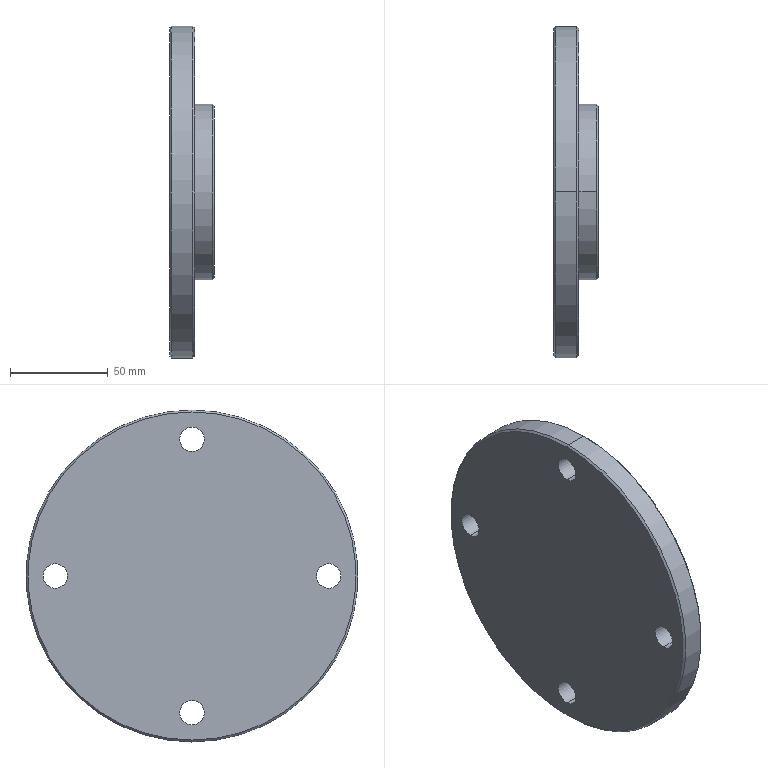Part | SolidWorks | features Chamfer 1, CirPattern 1, ICE 1, Revolution 1 | 1 solid | 26 faces | box 23 x 170 x 170 mm | volume 323268 mm3 | cylinder 14 | cone 8 | plane 4 | commonest cylinder face diameters 12.5 x8 60 x2 90 x2 170 x2
STEP:
#1=CARTESIAN_POINT('',(13.,0.,-84.));
#2=VERTEX_POINT('',#1);
#3=CARTESIAN_POINT('',(13.,0.,84.));
#4=VERTEX_POINT('',#3);
#5=CARTESIAN_POINT('',(13.,0.,0.));
#6=DIRECTION('',(1.,0.,0.));
#7=DIRECTION('',(0.,0.,1.));
#8=AXIS2_PLACEMENT_3D('',#5,#6,#7);
#9=CIRCLE('',#8,84.);
#10=EDGE_CURVE('',#2,#4,#9,.T.);
#11=ORIENTED_EDGE('',*,*,#10,.F.);
#12=CARTESIAN_POINT('',(12.,0.,-85.));
#13=VERTEX_POINT('',#12);
#14=CARTESIAN_POINT('',(12.,0.,-85.));
#15=DIRECTION('',(-0.7071,0.,-0.7071));
#16=VECTOR('',#15,1000.);
#17=LINE('',#14,#16);
#18=EDGE_CURVE('',#2,#13,#17,.T.);
#19=ORIENTED_EDGE('',*,*,#18,.T.);
#20=CARTESIAN_POINT('',(12.,0.,85.));
#21=VERTEX_POINT('',#20);
#22=CARTESIAN_POINT('',(12.,0.,0.));
#23=DIRECTION('',(-1.,0.,0.));
#24=DIRECTION('',(0.,0.,1.));
#25=AXIS2_PLACEMENT_3D('',#22,#23,#24);
#26=CIRCLE('',#25,85.);
#27=EDGE_CURVE('',#21,#13,#26,.T.);
#28=ORIENTED_EDGE('',*,*,#27,.F.);
#29=CARTESIAN_POINT('',(12.,0.,85.));
#30=DIRECTION('',(-0.7071,0.,0.7071));
#31=VECTOR('',#30,1000.);
#32=LINE('',#29,#31);
#33=EDGE_CURVE('',#4,#21,#32,.T.);
#34=ORIENTED_EDGE('',*,*,#33,.F.);
#35=EDGE_LOOP('',(#11,#19,#28,#34));
#36=FACE_OUTER_BOUND('',#35,.T.);
#37=CARTESIAN_POINT('',(12.,0.,0.));
#38=DIRECTION('',(-1.,0.,0.));
#39=DIRECTION('',(0.,0.,1.));
#40=AXIS2_PLACEMENT_3D('',#37,#38,#39);
#41=CONICAL_SURFACE('',#40,85.,0.7854);
#42=ADVANCED_FACE('',(#36),#41,.T.);
#43=CARTESIAN_POINT('',(0.,0.,84.));
#44=VERTEX_POINT('',#43);
#45=CARTESIAN_POINT('',(0.,0.,-84.));
#46=VERTEX_POINT('',#45);
#47=CARTESIAN_POINT('',(0.,0.,0.));
#48=DIRECTION('',(-1.,0.,0.));
#49=DIRECTION('',(0.,0.,-1.));
#50=AXIS2_PLACEMENT_3D('',#47,#48,#49);
#51=CIRCLE('',#50,84.);
#52=EDGE_CURVE('',#44,#46,#51,.T.);
#53=ORIENTED_EDGE('',*,*,#52,.F.);
#54=CARTESIAN_POINT('',(1.,0.,85.));
#55=VERTEX_POINT('',#54);
#56=CARTESIAN_POINT('',(0.,0.,84.));
#57=DIRECTION('',(0.7071,0.,0.7071));
#58=VECTOR('',#57,1000.);
#59=LINE('',#56,#58);
#60=EDGE_CURVE('',#44,#55,#59,.T.);
#61=ORIENTED_EDGE('',*,*,#60,.T.);
#62=CARTESIAN_POINT('',(1.,0.,-85.));
#63=VERTEX_POINT('',#62);
#64=CARTESIAN_POINT('',(1.,0.,0.));
#65=DIRECTION('',(1.,0.,0.));
#66=DIRECTION('',(0.,0.,-1.));
#67=AXIS2_PLACEMENT_3D('',#64,#65,#66);
#68=CIRCLE('',#67,85.);
#69=EDGE_CURVE('',#63,#55,#68,.T.);
#70=ORIENTED_EDGE('',*,*,#69,.F.);
#71=CARTESIAN_POINT('',(0.,0.,-84.));
#72=DIRECTION('',(0.7071,0.,-0.7071));
#73=VECTOR('',#72,1000.);
#74=LINE('',#71,#73);
#75=EDGE_CURVE('',#46,#63,#74,.T.);
#76=ORIENTED_EDGE('',*,*,#75,.F.);
#77=EDGE_LOOP('',(#53,#61,#70,#76));
#78=FACE_OUTER_BOUND('',#77,.T.);
#79=CARTESIAN_POINT('',(0.,0.,0.));
#80=DIRECTION('',(1.,0.,0.));
#81=DIRECTION('',(0.,0.,-1.));
#82=AXIS2_PLACEMENT_3D('',#79,#80,#81);
#83=CONICAL_SURFACE('',#82,84.,0.7854);
#84=ADVANCED_FACE('',(#78),#83,.T.);
#85=CARTESIAN_POINT('',(23.,0.,-44.));
#86=VERTEX_POINT('',#85);
#87=CARTESIAN_POINT('',(23.,0.,44.));
#88=VERTEX_POINT('',#87);
#89=CARTESIAN_POINT('',(23.,0.,0.));
#90=DIRECTION('',(1.,0.,0.));
#91=DIRECTION('',(0.,0.,1.));
#92=AXIS2_PLACEMENT_3D('',#89,#90,#91);
#93=CIRCLE('',#92,44.);
#94=EDGE_CURVE('',#86,#88,#93,.T.);
#95=ORIENTED_EDGE('',*,*,#94,.F.);
#96=CARTESIAN_POINT('',(22.,0.,-45.));
#97=VERTEX_POINT('',#96);
#98=CARTESIAN_POINT('',(22.,0.,-45.));
#99=DIRECTION('',(-0.7071,0.,-0.7071));
#100=VECTOR('',#99,1000.);
#101=LINE('',#98,#100);
#102=EDGE_CURVE('',#86,#97,#101,.T.);
#103=ORIENTED_EDGE('',*,*,#102,.T.);
#104=CARTESIAN_POINT('',(22.,0.,45.));
#105=VERTEX_POINT('',#104);
#106=CARTESIAN_POINT('',(22.,0.,0.));
#107=DIRECTION('',(-1.,0.,0.));
#108=DIRECTION('',(0.,0.,1.));
#109=AXIS2_PLACEMENT_3D('',#106,#107,#108);
#110=CIRCLE('',#109,45.);
#111=EDGE_CURVE('',#105,#97,#110,.T.);
#112=ORIENTED_EDGE('',*,*,#111,.F.);
#113=CARTESIAN_POINT('',(22.,0.,45.));
#114=DIRECTION('',(-0.7071,0.,0.7071));
#115=VECTOR('',#114,1000.);
#116=LINE('',#113,#115);
#117=EDGE_CURVE('',#88,#105,#116,.T.);
#118=ORIENTED_EDGE('',*,*,#117,.F.);
#119=EDGE_LOOP('',(#95,#103,#112,#118));
#120=FACE_OUTER_BOUND('',#119,.T.);
#121=CARTESIAN_POINT('',(22.,0.,0.));
#122=DIRECTION('',(-1.,0.,0.));
#123=DIRECTION('',(0.,0.,1.));
#124=AXIS2_PLACEMENT_3D('',#121,#122,#123);
#125=CONICAL_SURFACE('',#124,45.,0.7854);
#126=ADVANCED_FACE('',(#120),#125,.T.);
#127=CARTESIAN_POINT('',(22.,0.,30.));
#128=VERTEX_POINT('',#127);
#129=CARTESIAN_POINT('',(22.,0.,-30.));
#130=VERTEX_POINT('',#129);
#131=CARTESIAN_POINT('',(22.,0.,0.));
#132=DIRECTION('',(1.,0.,0.));
#133=DIRECTION('',(0.,0.,1.));
#134=AXIS2_PLACEMENT_3D('',#131,#132,#133);
#135=CIRCLE('',#134,30.);
#136=EDGE_CURVE('',#128,#130,#135,.T.);
#137=ORIENTED_EDGE('',*,*,#136,.F.);
#138=CARTESIAN_POINT('',(23.,0.,31.));
#139=VERTEX_POINT('',#138);
#140=CARTESIAN_POINT('',(23.,0.,31.));
#141=DIRECTION('',(0.7071,0.,0.7071));
#142=VECTOR('',#141,1000.);
#143=LINE('',#140,#142);
#144=EDGE_CURVE('',#128,#139,#143,.T.);
#145=ORIENTED_EDGE('',*,*,#144,.T.);
#146=CARTESIAN_POINT('',(23.,0.,-31.));
#147=VERTEX_POINT('',#146);
#148=CARTESIAN_POINT('',(23.,0.,0.));
#149=DIRECTION('',(-1.,0.,0.));
#150=DIRECTION('',(0.,0.,1.));
#151=AXIS2_PLACEMENT_3D('',#148,#149,#150);
#152=CIRCLE('',#151,31.);
#153=EDGE_CURVE('',#147,#139,#152,.T.);
#154=ORIENTED_EDGE('',*,*,#153,.F.);
#155=CARTESIAN_POINT('',(23.,0.,-31.));
#156=DIRECTION('',(0.7071,0.,-0.7071));
#157=VECTOR('',#156,1000.);
#158=LINE('',#155,#157);
#159=EDGE_CURVE('',#130,#147,#158,.T.);
#160=ORIENTED_EDGE('',*,*,#159,.F.);
#161=EDGE_LOOP('',(#137,#145,#154,#160));
#162=FACE_OUTER_BOUND('',#161,.T.);
#163=CARTESIAN_POINT('',(23.,0.,0.));
#164=DIRECTION('',(1.,0.,0.));
#165=DIRECTION('',(0.,0.,-1.));
#166=AXIS2_PLACEMENT_3D('',#163,#164,#165);
#167=CONICAL_SURFACE('',#166,31.,0.7854);
#168=ADVANCED_FACE('',(#162),#167,.F.);
#169=CARTESIAN_POINT('',(13.,-70.,-6.25));
#170=VERTEX_POINT('',#169);
#171=CARTESIAN_POINT('',(13.,-70.,6.25));
#172=VERTEX_POINT('',#171);
#173=CARTESIAN_POINT('',(13.,-70.,0.));
#174=DIRECTION('',(-1.,0.,0.));
#175=DIRECTION('',(0.,0.,1.));
#176=AXIS2_PLACEMENT_3D('',#173,#174,#175);
#177=CIRCLE('',#176,6.25);
#178=EDGE_CURVE('',#170,#172,#177,.T.);
#179=ORIENTED_EDGE('',*,*,#178,.F.);
#180=CARTESIAN_POINT('',(0.,-70.,-6.25));
#181=VERTEX_POINT('',#180);
#182=CARTESIAN_POINT('',(23.,-70.,-6.25));
#183=DIRECTION('',(-1.,0.,0.));
#184=VECTOR('',#183,1000.);
#185=LINE('',#182,#184);
#186=EDGE_CURVE('',#170,#181,#185,.T.);
#187=ORIENTED_EDGE('',*,*,#186,.T.);
#188=CARTESIAN_POINT('',(0.,-70.,6.25));
#189=VERTEX_POINT('',#188);
#190=CARTESIAN_POINT('',(0.,-70.,0.));
#191=DIRECTION('',(-1.,0.,0.));
#192=DIRECTION('',(0.,0.,-1.));
#193=AXIS2_PLACEMENT_3D('',#190,#191,#192);
#194=CIRCLE('',#193,6.25);
#195=EDGE_CURVE('',#181,#189,#194,.T.);
#196=ORIENTED_EDGE('',*,*,#195,.T.);
#197=CARTESIAN_POINT('',(23.,-70.,6.25));
#198=DIRECTION('',(-1.,0.,0.));
#199=VECTOR('',#198,1000.);
#200=LINE('',#197,#199);
#201=EDGE_CURVE('',#172,#189,#200,.T.);
#202=ORIENTED_EDGE('',*,*,#201,.F.);
#203=EDGE_LOOP('',(#179,#187,#196,#202));
#204=FACE_OUTER_BOUND('',#203,.T.);
#205=CARTESIAN_POINT('',(23.,-70.,0.));
#206=DIRECTION('',(-1.,0.,0.));
#207=DIRECTION('',(0.,0.,1.));
#208=AXIS2_PLACEMENT_3D('',#205,#206,#207);
#209=CYLINDRICAL_SURFACE('',#208,6.25);
#210=ADVANCED_FACE('',(#204),#209,.F.);
#211=CARTESIAN_POINT('',(13.,0.,63.75));
#212=VERTEX_POINT('',#211);
#213=CARTESIAN_POINT('',(13.,0.,76.25));
#214=VERTEX_POINT('',#213);
#215=CARTESIAN_POINT('',(13.,0.,70.));
#216=DIRECTION('',(-1.,0.,0.));
#217=DIRECTION('',(0.,0.,1.));
#218=AXIS2_PLACEMENT_3D('',#215,#216,#217);
#219=CIRCLE('',#218,6.25);
#220=EDGE_CURVE('',#212,#214,#219,.T.);
#221=ORIENTED_EDGE('',*,*,#220,.F.);
#222=CARTESIAN_POINT('',(0.,0.,63.75));
#223=VERTEX_POINT('',#222);
#224=CARTESIAN_POINT('',(23.,0.,63.75));
#225=DIRECTION('',(-1.,0.,0.));
#226=VECTOR('',#225,1000.);
#227=LINE('',#224,#226);
#228=EDGE_CURVE('',#212,#223,#227,.T.);
#229=ORIENTED_EDGE('',*,*,#228,.T.);
#230=CARTESIAN_POINT('',(0.,0.,76.25));
#231=VERTEX_POINT('',#230);
#232=CARTESIAN_POINT('',(0.,0.,70.));
#233=DIRECTION('',(-1.,0.,0.));
#234=DIRECTION('',(0.,-1.,0.));
#235=AXIS2_PLACEMENT_3D('',#232,#233,#234);
#236=CIRCLE('',#235,6.25);
#237=EDGE_CURVE('',#223,#231,#236,.T.);
#238=ORIENTED_EDGE('',*,*,#237,.T.);
#239=CARTESIAN_POINT('',(23.,0.,76.25));
#240=DIRECTION('',(-1.,0.,0.));
#241=VECTOR('',#240,1000.);
#242=LINE('',#239,#241);
#243=EDGE_CURVE('',#214,#231,#242,.T.);
#244=ORIENTED_EDGE('',*,*,#243,.F.);
#245=EDGE_LOOP('',(#221,#229,#238,#244));
#246=FACE_OUTER_BOUND('',#245,.T.);
#247=CARTESIAN_POINT('',(23.,0.,70.));
#248=DIRECTION('',(-1.,0.,0.));
#249=DIRECTION('',(0.,0.,1.));
#250=AXIS2_PLACEMENT_3D('',#247,#248,#249);
#251=CYLINDRICAL_SURFACE('',#250,6.25);
#252=ADVANCED_FACE('',(#246),#251,.F.);
#253=CARTESIAN_POINT('',(13.,0.,-76.25));
#254=VERTEX_POINT('',#253);
#255=CARTESIAN_POINT('',(13.,0.,-63.75));
#256=VERTEX_POINT('',#255);
#257=CARTESIAN_POINT('',(13.,0.,-70.));
#258=DIRECTION('',(-1.,0.,0.));
#259=DIRECTION('',(0.,0.,1.));
#260=AXIS2_PLACEMENT_3D('',#257,#258,#259);
#261=CIRCLE('',#260,6.25);
#262=EDGE_CURVE('',#254,#256,#261,.T.);
#263=ORIENTED_EDGE('',*,*,#262,.F.);
#264=CARTESIAN_POINT('',(0.,0.,-76.25));
#265=VERTEX_POINT('',#264);
#266=CARTESIAN_POINT('',(23.,0.,-76.25));
#267=DIRECTION('',(-1.,0.,0.));
#268=VECTOR('',#267,1000.);
#269=LINE('',#266,#268);
#270=EDGE_CURVE('',#254,#265,#269,.T.);
#271=ORIENTED_EDGE('',*,*,#270,.T.);
#272=CARTESIAN_POINT('',(0.,0.,-63.75));
#273=VERTEX_POINT('',#272);
#274=CARTESIAN_POINT('',(0.,0.,-70.));
#275=DIRECTION('',(-1.,0.,0.));
#276=DIRECTION('',(0.,1.,0.));
#277=AXIS2_PLACEMENT_3D('',#274,#275,#276);
#278=CIRCLE('',#277,6.25);
#279=EDGE_CURVE('',#265,#273,#278,.T.);
#280=ORIENTED_EDGE('',*,*,#279,.T.);
#281=CARTESIAN_POINT('',(23.,0.,-63.75));
#282=DIRECTION('',(-1.,0.,0.));
#283=VECTOR('',#282,1000.);
#284=LINE('',#281,#283);
#285=EDGE_CURVE('',#256,#273,#284,.T.);
#286=ORIENTED_EDGE('',*,*,#285,.F.);
#287=EDGE_LOOP('',(#263,#271,#280,#286));
#288=FACE_OUTER_BOUND('',#287,.T.);
#289=CARTESIAN_POINT('',(23.,0.,-70.));
#290=DIRECTION('',(-1.,0.,0.));
#291=DIRECTION('',(0.,0.,1.));
#292=AXIS2_PLACEMENT_3D('',#289,#290,#291);
#293=CYLINDRICAL_SURFACE('',#292,6.25);
#294=ADVANCED_FACE('',(#288),#293,.F.);
#295=CARTESIAN_POINT('',(13.,70.,-6.25));
#296=VERTEX_POINT('',#295);
#297=CARTESIAN_POINT('',(13.,70.,6.25));
#298=VERTEX_POINT('',#297);
#299=CARTESIAN_POINT('',(13.,70.,0.));
#300=DIRECTION('',(-1.,0.,0.));
#301=DIRECTION('',(0.,0.,1.));
#302=AXIS2_PLACEMENT_3D('',#299,#300,#301);
#303=CIRCLE('',#302,6.25);
#304=EDGE_CURVE('',#296,#298,#303,.T.);
#305=ORIENTED_EDGE('',*,*,#304,.F.);
#306=CARTESIAN_POINT('',(0.,70.,-6.25));
#307=VERTEX_POINT('',#306);
#308=CARTESIAN_POINT('',(23.,70.,-6.25));
#309=DIRECTION('',(-1.,0.,0.));
#310=VECTOR('',#309,1000.);
#311=LINE('',#308,#310);
#312=EDGE_CURVE('',#296,#307,#311,.T.);
#313=ORIENTED_EDGE('',*,*,#312,.T.);
#314=CARTESIAN_POINT('',(0.,70.,6.25));
#315=VERTEX_POINT('',#314);
#316=CARTESIAN_POINT('',(0.,70.,0.));
#317=DIRECTION('',(-1.,0.,0.));
#318=DIRECTION('',(0.,0.,1.));
#319=AXIS2_PLACEMENT_3D('',#316,#317,#318);
#320=CIRCLE('',#319,6.25);
#321=EDGE_CURVE('',#307,#315,#320,.T.);
#322=ORIENTED_EDGE('',*,*,#321,.T.);
#323=CARTESIAN_POINT('',(23.,70.,6.25));
#324=DIRECTION('',(-1.,0.,0.));
#325=VECTOR('',#324,1000.);
#326=LINE('',#323,#325);
#327=EDGE_CURVE('',#298,#315,#326,.T.);
#328=ORIENTED_EDGE('',*,*,#327,.F.);
#329=EDGE_LOOP('',(#305,#313,#322,#328));
#330=FACE_OUTER_BOUND('',#329,.T.);
#331=CARTESIAN_POINT('',(23.,70.,0.));
#332=DIRECTION('',(-1.,0.,0.));
#333=DIRECTION('',(0.,0.,1.));
#334=AXIS2_PLACEMENT_3D('',#331,#332,#333);
#335=CYLINDRICAL_SURFACE('',#334,6.25);
#336=ADVANCED_FACE('',(#330),#335,.F.);
#337=ORIENTED_EDGE('',*,*,#136,.T.);
#338=CARTESIAN_POINT('',(13.,0.,-30.));
#339=VERTEX_POINT('',#338);
#340=CARTESIAN_POINT('',(0.,0.,-30.));
#341=DIRECTION('',(-1.,0.,0.));
#342=VECTOR('',#341,1000.);
#343=LINE('',#340,#342);
#344=EDGE_CURVE('',#130,#339,#343,.T.);
#345=ORIENTED_EDGE('',*,*,#344,.T.);
#346=CARTESIAN_POINT('',(13.,0.,30.));
#347=VERTEX_POINT('',#346);
#348=CARTESIAN_POINT('',(13.,0.,0.));
#349=DIRECTION('',(-1.,0.,0.));
#350=DIRECTION('',(0.,0.,1.));
#351=AXIS2_PLACEMENT_3D('',#348,#349,#350);
#352=CIRCLE('',#351,30.);
#353=EDGE_CURVE('',#339,#347,#352,.T.);
#354=ORIENTED_EDGE('',*,*,#353,.T.);
#355=CARTESIAN_POINT('',(0.,0.,30.));
#356=DIRECTION('',(-1.,0.,0.));
#357=VECTOR('',#356,1000.);
#358=LINE('',#355,#357);
#359=EDGE_CURVE('',#128,#347,#358,.T.);
#360=ORIENTED_EDGE('',*,*,#359,.F.);
#361=EDGE_LOOP('',(#337,#345,#354,#360));
#362=FACE_OUTER_BOUND('',#361,.T.);
#363=CARTESIAN_POINT('',(0.,0.,0.));
#364=DIRECTION('',(-1.,0.,0.));
#365=DIRECTION('',(0.,0.,1.));
#366=AXIS2_PLACEMENT_3D('',#363,#364,#365);
#367=CYLINDRICAL_SURFACE('',#366,30.);
#368=ADVANCED_FACE('',(#362),#367,.F.);
#369=ORIENTED_EDGE('',*,*,#111,.T.);
#370=CARTESIAN_POINT('',(13.,0.,-45.));
#371=VERTEX_POINT('',#370);
#372=CARTESIAN_POINT('',(0.,0.,-45.));
#373=DIRECTION('',(-1.,0.,0.));
#374=VECTOR('',#373,1000.);
#375=LINE('',#372,#374);
#376=EDGE_CURVE('',#97,#371,#375,.T.);
#377=ORIENTED_EDGE('',*,*,#376,.T.);
#378=CARTESIAN_POINT('',(13.,0.,45.));
#379=VERTEX_POINT('',#378);
#380=CARTESIAN_POINT('',(13.,0.,0.));
#381=DIRECTION('',(-1.,0.,0.));
#382=DIRECTION('',(0.,0.,1.));
#383=AXIS2_PLACEMENT_3D('',#380,#381,#382);
#384=CIRCLE('',#383,45.);
#385=EDGE_CURVE('',#379,#371,#384,.T.);
#386=ORIENTED_EDGE('',*,*,#385,.F.);
#387=CARTESIAN_POINT('',(0.,0.,45.));
#388=DIRECTION('',(-1.,0.,0.));
#389=VECTOR('',#388,1000.);
#390=LINE('',#387,#389);
#391=EDGE_CURVE('',#105,#379,#390,.T.);
#392=ORIENTED_EDGE('',*,*,#391,.F.);
#393=EDGE_LOOP('',(#369,#377,#386,#392));
#394=FACE_OUTER_BOUND('',#393,.T.);
#395=CARTESIAN_POINT('',(0.,0.,0.));
#396=DIRECTION('',(-1.,0.,0.));
#397=DIRECTION('',(0.,0.,1.));
#398=AXIS2_PLACEMENT_3D('',#395,#396,#397);
#399=CYLINDRICAL_SURFACE('',#398,45.);
#400=ADVANCED_FACE('',(#394),#399,.T.);
#401=ORIENTED_EDGE('',*,*,#27,.T.);
#402=CARTESIAN_POINT('',(0.,0.,-85.));
#403=DIRECTION('',(-1.,0.,0.));
#404=VECTOR('',#403,1000.);
#405=LINE('',#402,#404);
#406=EDGE_CURVE('',#13,#63,#405,.T.);
#407=ORIENTED_EDGE('',*,*,#406,.T.);
#408=ORIENTED_EDGE('',*,*,#69,.T.);
#409=CARTESIAN_POINT('',(0.,0.,85.));
#410=DIRECTION('',(-1.,0.,0.));
#411=VECTOR('',#410,1000.);
#412=LINE('',#409,#411);
#413=EDGE_CURVE('',#21,#55,#412,.T.);
#414=ORIENTED_EDGE('',*,*,#413,.F.);
#415=EDGE_LOOP('',(#401,#407,#408,#414));
#416=FACE_OUTER_BOUND('',#415,.T.);
#417=CARTESIAN_POINT('',(0.,0.,0.));
#418=DIRECTION('',(-1.,0.,0.));
#419=DIRECTION('',(0.,0.,1.));
#420=AXIS2_PLACEMENT_3D('',#417,#418,#419);
#421=CYLINDRICAL_SURFACE('',#420,85.);
#422=ADVANCED_FACE('',(#416),#421,.T.);
#423=CARTESIAN_POINT('',(0.,0.,0.));
#424=DIRECTION('',(-1.,0.,0.));
#425=DIRECTION('',(0.,0.,-1.));
#426=AXIS2_PLACEMENT_3D('',#423,#424,#425);
#427=CIRCLE('',#426,84.);
#428=EDGE_CURVE('',#46,#44,#427,.T.);
#429=ORIENTED_EDGE('',*,*,#428,.T.);
#430=ORIENTED_EDGE('',*,*,#52,.T.);
#431=EDGE_LOOP('',(#429,#430));
#432=FACE_OUTER_BOUND('',#431,.T.);
#433=CARTESIAN_POINT('',(0.,-70.,0.));
#434=DIRECTION('',(-1.,0.,0.));
#435=DIRECTION('',(0.,0.,-1.));
#436=AXIS2_PLACEMENT_3D('',#433,#434,#435);
#437=CIRCLE('',#436,6.25);
#438=EDGE_CURVE('',#189,#181,#437,.T.);
#439=ORIENTED_EDGE('',*,*,#438,.F.);
#440=ORIENTED_EDGE('',*,*,#195,.F.);
#441=EDGE_LOOP('',(#439,#440));
#442=FACE_BOUND('',#441,.T.);
#443=CARTESIAN_POINT('',(0.,0.,70.));
#444=DIRECTION('',(-1.,0.,0.));
#445=DIRECTION('',(0.,-1.,0.));
#446=AXIS2_PLACEMENT_3D('',#443,#444,#445);
#447=CIRCLE('',#446,6.25);
#448=EDGE_CURVE('',#231,#223,#447,.T.);
#449=ORIENTED_EDGE('',*,*,#448,.F.);
#450=ORIENTED_EDGE('',*,*,#237,.F.);
#451=EDGE_LOOP('',(#449,#450));
#452=FACE_BOUND('',#451,.T.);
#453=CARTESIAN_POINT('',(0.,0.,-70.));
#454=DIRECTION('',(-1.,0.,0.));
#455=DIRECTION('',(0.,1.,0.));
#456=AXIS2_PLACEMENT_3D('',#453,#454,#455);
#457=CIRCLE('',#456,6.25);
#458=EDGE_CURVE('',#273,#265,#457,.T.);
#459=ORIENTED_EDGE('',*,*,#458,.F.);
#460=ORIENTED_EDGE('',*,*,#279,.F.);
#461=EDGE_LOOP('',(#459,#460));
#462=FACE_BOUND('',#461,.T.);
#463=CARTESIAN_POINT('',(0.,70.,0.));
#464=DIRECTION('',(-1.,0.,0.));
#465=DIRECTION('',(0.,0.,1.));
#466=AXIS2_PLACEMENT_3D('',#463,#464,#465);
#467=CIRCLE('',#466,6.25);
#468=EDGE_CURVE('',#315,#307,#467,.T.);
#469=ORIENTED_EDGE('',*,*,#468,.F.);
#470=ORIENTED_EDGE('',*,*,#321,.F.);
#471=EDGE_LOOP('',(#469,#470));
#472=FACE_BOUND('',#471,.T.);
#473=CARTESIAN_POINT('',(0.,0.,0.));
#474=DIRECTION('',(1.,0.,0.));
#475=DIRECTION('',(0.,0.,-1.));
#476=AXIS2_PLACEMENT_3D('',#473,#474,#475);
#477=PLANE('',#476);
#478=ADVANCED_FACE('',(#432,#442,#452,#462,#472),#477,.F.);
#479=ORIENTED_EDGE('',*,*,#406,.F.);
#480=CARTESIAN_POINT('',(12.,0.,0.));
#481=DIRECTION('',(-1.,0.,0.));
#482=DIRECTION('',(0.,0.,1.));
#483=AXIS2_PLACEMENT_3D('',#480,#481,#482);
#484=CIRCLE('',#483,85.);
#485=EDGE_CURVE('',#13,#21,#484,.T.);
#486=ORIENTED_EDGE('',*,*,#485,.T.);
#487=ORIENTED_EDGE('',*,*,#413,.T.);
#488=CARTESIAN_POINT('',(1.,0.,0.));
#489=DIRECTION('',(1.,0.,0.));
#490=DIRECTION('',(0.,0.,-1.));
#491=AXIS2_PLACEMENT_3D('',#488,#489,#490);
#492=CIRCLE('',#491,85.);
#493=EDGE_CURVE('',#55,#63,#492,.T.);
#494=ORIENTED_EDGE('',*,*,#493,.T.);
#495=EDGE_LOOP('',(#479,#486,#487,#494));
#496=FACE_OUTER_BOUND('',#495,.T.);
#497=CARTESIAN_POINT('',(0.,0.,0.));
#498=DIRECTION('',(-1.,0.,0.));
#499=DIRECTION('',(0.,0.,1.));
#500=AXIS2_PLACEMENT_3D('',#497,#498,#499);
#501=CYLINDRICAL_SURFACE('',#500,85.);
#502=ADVANCED_FACE('',(#496),#501,.T.);
#503=CARTESIAN_POINT('',(13.,0.,0.));
#504=DIRECTION('',(1.,0.,0.));
#505=DIRECTION('',(0.,0.,1.));
#506=AXIS2_PLACEMENT_3D('',#503,#504,#505);
#507=CIRCLE('',#506,84.);
#508=EDGE_CURVE('',#4,#2,#507,.T.);
#509=ORIENTED_EDGE('',*,*,#508,.T.);
#510=ORIENTED_EDGE('',*,*,#10,.T.);
#511=EDGE_LOOP('',(#509,#510));
#512=FACE_OUTER_BOUND('',#511,.T.);
#513=CARTESIAN_POINT('',(13.,-70.,0.));
#514=DIRECTION('',(-1.,0.,0.));
#515=DIRECTION('',(0.,0.,1.));
#516=AXIS2_PLACEMENT_3D('',#513,#514,#515);
#517=CIRCLE('',#516,6.25);
#518=EDGE_CURVE('',#172,#170,#517,.T.);
#519=ORIENTED_EDGE('',*,*,#518,.T.);
#520=ORIENTED_EDGE('',*,*,#178,.T.);
#521=EDGE_LOOP('',(#519,#520));
#522=FACE_BOUND('',#521,.T.);
#523=CARTESIAN_POINT('',(13.,0.,70.));
#524=DIRECTION('',(-1.,0.,0.));
#525=DIRECTION('',(0.,0.,1.));
#526=AXIS2_PLACEMENT_3D('',#523,#524,#525);
#527=CIRCLE('',#526,6.25);
#528=EDGE_CURVE('',#214,#212,#527,.T.);
#529=ORIENTED_EDGE('',*,*,#528,.T.);
#530=ORIENTED_EDGE('',*,*,#220,.T.);
#531=EDGE_LOOP('',(#529,#530));
#532=FACE_BOUND('',#531,.T.);
#533=CARTESIAN_POINT('',(13.,0.,-70.));
#534=DIRECTION('',(-1.,0.,0.));
#535=DIRECTION('',(0.,0.,1.));
#536=AXIS2_PLACEMENT_3D('',#533,#534,#535);
#537=CIRCLE('',#536,6.25);
#538=EDGE_CURVE('',#256,#254,#537,.T.);
#539=ORIENTED_EDGE('',*,*,#538,.T.);
#540=ORIENTED_EDGE('',*,*,#262,.T.);
#541=EDGE_LOOP('',(#539,#540));
#542=FACE_BOUND('',#541,.T.);
#543=CARTESIAN_POINT('',(13.,70.,0.));
#544=DIRECTION('',(-1.,0.,0.));
#545=DIRECTION('',(0.,0.,1.));
#546=AXIS2_PLACEMENT_3D('',#543,#544,#545);
#547=CIRCLE('',#546,6.25);
#548=EDGE_CURVE('',#298,#296,#547,.T.);
#549=ORIENTED_EDGE('',*,*,#548,.T.);
#550=ORIENTED_EDGE('',*,*,#304,.T.);
#551=EDGE_LOOP('',(#549,#550));
#552=FACE_BOUND('',#551,.T.);
#553=ORIENTED_EDGE('',*,*,#385,.T.);
#554=CARTESIAN_POINT('',(13.,0.,0.));
#555=DIRECTION('',(-1.,0.,0.));
#556=DIRECTION('',(0.,0.,1.));
#557=AXIS2_PLACEMENT_3D('',#554,#555,#556);
#558=CIRCLE('',#557,45.);
#559=EDGE_CURVE('',#371,#379,#558,.T.);
#560=ORIENTED_EDGE('',*,*,#559,.T.);
#561=EDGE_LOOP('',(#553,#560));
#562=FACE_BOUND('',#561,.T.);
#563=CARTESIAN_POINT('',(13.,85.,0.));
#564=DIRECTION('',(-1.,0.,0.));
#565=DIRECTION('',(0.,0.,1.));
#566=AXIS2_PLACEMENT_3D('',#563,#564,#565);
#567=PLANE('',#566);
#568=ADVANCED_FACE('',(#512,#522,#532,#542,#552,#562),#567,.F.);
#569=ORIENTED_EDGE('',*,*,#376,.F.);
#570=CARTESIAN_POINT('',(22.,0.,0.));
#571=DIRECTION('',(-1.,0.,0.));
#572=DIRECTION('',(0.,0.,1.));
#573=AXIS2_PLACEMENT_3D('',#570,#571,#572);
#574=CIRCLE('',#573,45.);
#575=EDGE_CURVE('',#97,#105,#574,.T.);
#576=ORIENTED_EDGE('',*,*,#575,.T.);
#577=ORIENTED_EDGE('',*,*,#391,.T.);
#578=ORIENTED_EDGE('',*,*,#559,.F.);
#579=EDGE_LOOP('',(#569,#576,#577,#578));
#580=FACE_OUTER_BOUND('',#579,.T.);
#581=CARTESIAN_POINT('',(0.,0.,0.));
#582=DIRECTION('',(-1.,0.,0.));
#583=DIRECTION('',(0.,0.,1.));
#584=AXIS2_PLACEMENT_3D('',#581,#582,#583);
#585=CYLINDRICAL_SURFACE('',#584,45.);
#586=ADVANCED_FACE('',(#580),#585,.T.);
#587=ORIENTED_EDGE('',*,*,#153,.T.);
#588=CARTESIAN_POINT('',(23.,0.,0.));
#589=DIRECTION('',(-1.,0.,0.));
#590=DIRECTION('',(0.,0.,1.));
#591=AXIS2_PLACEMENT_3D('',#588,#589,#590);
#592=CIRCLE('',#591,31.);
#593=EDGE_CURVE('',#139,#147,#592,.T.);
#594=ORIENTED_EDGE('',*,*,#593,.T.);
#595=EDGE_LOOP('',(#587,#594));
#596=FACE_BOUND('',#595,.T.);
#597=CARTESIAN_POINT('',(23.,0.,0.));
#598=DIRECTION('',(1.,0.,0.));
#599=DIRECTION('',(0.,0.,1.));
#600=AXIS2_PLACEMENT_3D('',#597,#598,#599);
#601=CIRCLE('',#600,44.);
#602=EDGE_CURVE('',#88,#86,#601,.T.);
#603=ORIENTED_EDGE('',*,*,#602,.T.);
#604=ORIENTED_EDGE('',*,*,#94,.T.);
#605=EDGE_LOOP('',(#603,#604));
#606=FACE_OUTER_BOUND('',#605,.T.);
#607=CARTESIAN_POINT('',(23.,45.,0.));
#608=DIRECTION('',(-1.,0.,0.));
#609=DIRECTION('',(0.,0.,1.));
#610=AXIS2_PLACEMENT_3D('',#607,#608,#609);
#611=PLANE('',#610);
#612=ADVANCED_FACE('',(#596,#606),#611,.F.);
#613=ORIENTED_EDGE('',*,*,#344,.F.);
#614=CARTESIAN_POINT('',(22.,0.,0.));
#615=DIRECTION('',(1.,0.,0.));
#616=DIRECTION('',(0.,0.,1.));
#617=AXIS2_PLACEMENT_3D('',#614,#615,#616);
#618=CIRCLE('',#617,30.);
#619=EDGE_CURVE('',#130,#128,#618,.T.);
#620=ORIENTED_EDGE('',*,*,#619,.T.);
#621=ORIENTED_EDGE('',*,*,#359,.T.);
#622=CARTESIAN_POINT('',(13.,0.,0.));
#623=DIRECTION('',(-1.,0.,0.));
#624=DIRECTION('',(0.,0.,1.));
#625=AXIS2_PLACEMENT_3D('',#622,#623,#624);
#626=CIRCLE('',#625,30.);
#627=EDGE_CURVE('',#347,#339,#626,.T.);
#628=ORIENTED_EDGE('',*,*,#627,.T.);
#629=EDGE_LOOP('',(#613,#620,#621,#628));
#630=FACE_OUTER_BOUND('',#629,.T.);
#631=CARTESIAN_POINT('',(0.,0.,0.));
#632=DIRECTION('',(-1.,0.,0.));
#633=DIRECTION('',(0.,0.,1.));
#634=AXIS2_PLACEMENT_3D('',#631,#632,#633);
#635=CYLINDRICAL_SURFACE('',#634,30.);
#636=ADVANCED_FACE('',(#630),#635,.F.);
#637=ORIENTED_EDGE('',*,*,#627,.F.);
#638=ORIENTED_EDGE('',*,*,#353,.F.);
#639=EDGE_LOOP('',(#637,#638));
#640=FACE_OUTER_BOUND('',#639,.T.);
#641=CARTESIAN_POINT('',(13.,30.,0.));
#642=DIRECTION('',(-1.,0.,0.));
#643=DIRECTION('',(0.,0.,1.));
#644=AXIS2_PLACEMENT_3D('',#641,#642,#643);
#645=PLANE('',#644);
#646=ADVANCED_FACE('',(#640),#645,.F.);
#647=ORIENTED_EDGE('',*,*,#312,.F.);
#648=ORIENTED_EDGE('',*,*,#548,.F.);
#649=ORIENTED_EDGE('',*,*,#327,.T.);
#650=ORIENTED_EDGE('',*,*,#468,.T.);
#651=EDGE_LOOP('',(#647,#648,#649,#650));
#652=FACE_OUTER_BOUND('',#651,.T.);
#653=CARTESIAN_POINT('',(23.,70.,0.));
#654=DIRECTION('',(-1.,0.,0.));
#655=DIRECTION('',(0.,0.,1.));
#656=AXIS2_PLACEMENT_3D('',#653,#654,#655);
#657=CYLINDRICAL_SURFACE('',#656,6.25);
#658=ADVANCED_FACE('',(#652),#657,.F.);
#659=ORIENTED_EDGE('',*,*,#270,.F.);
#660=ORIENTED_EDGE('',*,*,#538,.F.);
#661=ORIENTED_EDGE('',*,*,#285,.T.);
#662=ORIENTED_EDGE('',*,*,#458,.T.);
#663=EDGE_LOOP('',(#659,#660,#661,#662));
#664=FACE_OUTER_BOUND('',#663,.T.);
#665=CARTESIAN_POINT('',(23.,0.,-70.));
#666=DIRECTION('',(-1.,0.,0.));
#667=DIRECTION('',(0.,0.,1.));
#668=AXIS2_PLACEMENT_3D('',#665,#666,#667);
#669=CYLINDRICAL_SURFACE('',#668,6.25);
#670=ADVANCED_FACE('',(#664),#669,.F.);
#671=ORIENTED_EDGE('',*,*,#228,.F.);
#672=ORIENTED_EDGE('',*,*,#528,.F.);
#673=ORIENTED_EDGE('',*,*,#243,.T.);
#674=ORIENTED_EDGE('',*,*,#448,.T.);
#675=EDGE_LOOP('',(#671,#672,#673,#674));
#676=FACE_OUTER_BOUND('',#675,.T.);
#677=CARTESIAN_POINT('',(23.,0.,70.));
#678=DIRECTION('',(-1.,0.,0.));
#679=DIRECTION('',(0.,0.,1.));
#680=AXIS2_PLACEMENT_3D('',#677,#678,#679);
#681=CYLINDRICAL_SURFACE('',#680,6.25);
#682=ADVANCED_FACE('',(#676),#681,.F.);
#683=ORIENTED_EDGE('',*,*,#186,.F.);
#684=ORIENTED_EDGE('',*,*,#518,.F.);
#685=ORIENTED_EDGE('',*,*,#201,.T.);
#686=ORIENTED_EDGE('',*,*,#438,.T.);
#687=EDGE_LOOP('',(#683,#684,#685,#686));
#688=FACE_OUTER_BOUND('',#687,.T.);
#689=CARTESIAN_POINT('',(23.,-70.,0.));
#690=DIRECTION('',(-1.,0.,0.));
#691=DIRECTION('',(0.,0.,1.));
#692=AXIS2_PLACEMENT_3D('',#689,#690,#691);
#693=CYLINDRICAL_SURFACE('',#692,6.25);
#694=ADVANCED_FACE('',(#688),#693,.F.);
#695=ORIENTED_EDGE('',*,*,#144,.F.);
#696=ORIENTED_EDGE('',*,*,#619,.F.);
#697=ORIENTED_EDGE('',*,*,#159,.T.);
#698=ORIENTED_EDGE('',*,*,#593,.F.);
#699=EDGE_LOOP('',(#695,#696,#697,#698));
#700=FACE_OUTER_BOUND('',#699,.T.);
#701=CARTESIAN_POINT('',(23.,0.,0.));
#702=DIRECTION('',(1.,0.,0.));
#703=DIRECTION('',(0.,0.,-1.));
#704=AXIS2_PLACEMENT_3D('',#701,#702,#703);
#705=CONICAL_SURFACE('',#704,31.,0.7854);
#706=ADVANCED_FACE('',(#700),#705,.F.);
#707=ORIENTED_EDGE('',*,*,#102,.F.);
#708=ORIENTED_EDGE('',*,*,#602,.F.);
#709=ORIENTED_EDGE('',*,*,#117,.T.);
#710=ORIENTED_EDGE('',*,*,#575,.F.);
#711=EDGE_LOOP('',(#707,#708,#709,#710));
#712=FACE_OUTER_BOUND('',#711,.T.);
#713=CARTESIAN_POINT('',(22.,0.,0.));
#714=DIRECTION('',(-1.,0.,0.));
#715=DIRECTION('',(0.,0.,1.));
#716=AXIS2_PLACEMENT_3D('',#713,#714,#715);
#717=CONICAL_SURFACE('',#716,45.,0.7854);
#718=ADVANCED_FACE('',(#712),#717,.T.);
#719=ORIENTED_EDGE('',*,*,#60,.F.);
#720=ORIENTED_EDGE('',*,*,#428,.F.);
#721=ORIENTED_EDGE('',*,*,#75,.T.);
#722=ORIENTED_EDGE('',*,*,#493,.F.);
#723=EDGE_LOOP('',(#719,#720,#721,#722));
#724=FACE_OUTER_BOUND('',#723,.T.);
#725=CARTESIAN_POINT('',(0.,0.,0.));
#726=DIRECTION('',(1.,0.,0.));
#727=DIRECTION('',(0.,0.,-1.));
#728=AXIS2_PLACEMENT_3D('',#725,#726,#727);
#729=CONICAL_SURFACE('',#728,84.,0.7854);
#730=ADVANCED_FACE('',(#724),#729,.T.);
#731=ORIENTED_EDGE('',*,*,#18,.F.);
#732=ORIENTED_EDGE('',*,*,#508,.F.);
#733=ORIENTED_EDGE('',*,*,#33,.T.);
#734=ORIENTED_EDGE('',*,*,#485,.F.);
#735=EDGE_LOOP('',(#731,#732,#733,#734));
#736=FACE_OUTER_BOUND('',#735,.T.);
#737=CARTESIAN_POINT('',(12.,0.,0.));
#738=DIRECTION('',(-1.,0.,0.));
#739=DIRECTION('',(0.,0.,1.));
#740=AXIS2_PLACEMENT_3D('',#737,#738,#739);
#741=CONICAL_SURFACE('',#740,85.,0.7854);
#742=ADVANCED_FACE('',(#736),#741,.T.);
#743=CLOSED_SHELL('',(#42,#84,#126,#168,#210,#252,#294,#336,#368,#400,#422,#478,#502,#568,#586,#612,#636,#646,#658,#670,#682,#694,#706,#718,#730,#742));
#744=MANIFOLD_SOLID_BREP('',#743);
#745=CARTESIAN_POINT('',(0.,0.,0.));
#746=DIRECTION('',(0.,0.,1.));
#747=DIRECTION('',(1.,0.,0.));
#748=AXIS2_PLACEMENT_3D('',#745,#746,#747);
#749=(LENGTH_UNIT()NAMED_UNIT(*)SI_UNIT(.MILLI.,.METRE.));
#750=UNCERTAINTY_MEASURE_WITH_UNIT(LENGTH_MEASURE(0.00001),#749,'','');
#751=(NAMED_UNIT(*)PLANE_ANGLE_UNIT()SI_UNIT($,.RADIAN.));
#752=(NAMED_UNIT(*)SI_UNIT($,.STERADIAN.)SOLID_ANGLE_UNIT());
#753=(GEOMETRIC_REPRESENTATION_CONTEXT(3)GLOBAL_UNCERTAINTY_ASSIGNED_CONTEXT((#750))GLOBAL_UNIT_ASSIGNED_CONTEXT((#749,#751,#752))REPRESENTATION_CONTEXT('',''));
#754=ADVANCED_BREP_SHAPE_REPRESENTATION('',(#744,#748),#753);